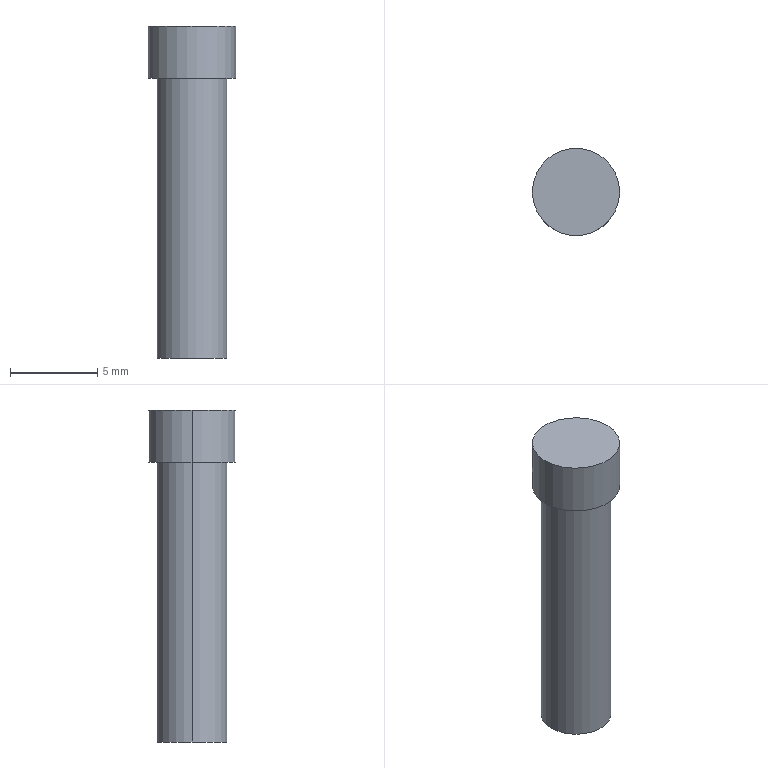Part | SolidWorks | features BaseBody 1 | 1 solid | 7 faces | box 5 x 5 x 19 mm | volume 259.967 mm3 | cylinder 4 | plane 3 | commonest cylinder face diameters 4 x2 5 x2
STEP:
#1=CARTESIAN_POINT('',(2.,0.,-5.5));
#2=VERTEX_POINT('',#1);
#3=CARTESIAN_POINT('',(-2.,0.,-5.5));
#4=VERTEX_POINT('',#3);
#5=CARTESIAN_POINT('',(0.,0.,-5.5));
#6=DIRECTION('',(0.,0.,1.));
#7=DIRECTION('',(1.,0.,0.));
#8=AXIS2_PLACEMENT_3D('',#5,#6,#7);
#9=CIRCLE('',#8,2.);
#10=EDGE_CURVE('',#2,#4,#9,.T.);
#11=ORIENTED_EDGE('',*,*,#10,.T.);
#12=CARTESIAN_POINT('',(-2.,0.,10.5));
#13=VERTEX_POINT('',#12);
#14=CARTESIAN_POINT('',(-2.,0.,-5.5));
#15=DIRECTION('',(0.,0.,1.));
#16=VECTOR('',#15,1000.);
#17=LINE('',#14,#16);
#18=EDGE_CURVE('',#4,#13,#17,.T.);
#19=ORIENTED_EDGE('',*,*,#18,.T.);
#20=CARTESIAN_POINT('',(2.,0.,10.5));
#21=VERTEX_POINT('',#20);
#22=CARTESIAN_POINT('',(0.,0.,10.5));
#23=DIRECTION('',(0.,0.,-1.));
#24=DIRECTION('',(1.,0.,0.));
#25=AXIS2_PLACEMENT_3D('',#22,#23,#24);
#26=CIRCLE('',#25,2.);
#27=EDGE_CURVE('',#13,#21,#26,.T.);
#28=ORIENTED_EDGE('',*,*,#27,.T.);
#29=CARTESIAN_POINT('',(2.,0.,-5.5));
#30=DIRECTION('',(0.,0.,1.));
#31=VECTOR('',#30,1000.);
#32=LINE('',#29,#31);
#33=EDGE_CURVE('',#2,#21,#32,.T.);
#34=ORIENTED_EDGE('',*,*,#33,.F.);
#35=EDGE_LOOP('',(#11,#19,#28,#34));
#36=FACE_OUTER_BOUND('',#35,.T.);
#37=CARTESIAN_POINT('',(0.,0.,-5.5));
#38=DIRECTION('',(0.,0.,1.));
#39=DIRECTION('',(1.,0.,0.));
#40=AXIS2_PLACEMENT_3D('',#37,#38,#39);
#41=CYLINDRICAL_SURFACE('',#40,2.);
#42=ADVANCED_FACE('',(#36),#41,.T.);
#43=CARTESIAN_POINT('',(2.5,0.,10.5));
#44=VERTEX_POINT('',#43);
#45=CARTESIAN_POINT('',(-2.5,0.,10.5));
#46=VERTEX_POINT('',#45);
#47=CARTESIAN_POINT('',(0.,0.,10.5));
#48=DIRECTION('',(0.,0.,1.));
#49=DIRECTION('',(1.,0.,0.));
#50=AXIS2_PLACEMENT_3D('',#47,#48,#49);
#51=CIRCLE('',#50,2.5);
#52=EDGE_CURVE('',#44,#46,#51,.T.);
#53=ORIENTED_EDGE('',*,*,#52,.T.);
#54=CARTESIAN_POINT('',(-2.5,0.,13.5));
#55=VERTEX_POINT('',#54);
#56=CARTESIAN_POINT('',(-2.5,0.,10.5));
#57=DIRECTION('',(0.,0.,1.));
#58=VECTOR('',#57,1000.);
#59=LINE('',#56,#58);
#60=EDGE_CURVE('',#46,#55,#59,.T.);
#61=ORIENTED_EDGE('',*,*,#60,.T.);
#62=CARTESIAN_POINT('',(2.5,0.,13.5));
#63=VERTEX_POINT('',#62);
#64=CARTESIAN_POINT('',(0.,0.,13.5));
#65=DIRECTION('',(0.,0.,-1.));
#66=DIRECTION('',(1.,0.,0.));
#67=AXIS2_PLACEMENT_3D('',#64,#65,#66);
#68=CIRCLE('',#67,2.5);
#69=EDGE_CURVE('',#55,#63,#68,.T.);
#70=ORIENTED_EDGE('',*,*,#69,.T.);
#71=CARTESIAN_POINT('',(2.5,0.,10.5));
#72=DIRECTION('',(0.,0.,1.));
#73=VECTOR('',#72,1000.);
#74=LINE('',#71,#73);
#75=EDGE_CURVE('',#44,#63,#74,.T.);
#76=ORIENTED_EDGE('',*,*,#75,.F.);
#77=EDGE_LOOP('',(#53,#61,#70,#76));
#78=FACE_OUTER_BOUND('',#77,.T.);
#79=CARTESIAN_POINT('',(0.,0.,10.5));
#80=DIRECTION('',(0.,0.,1.));
#81=DIRECTION('',(1.,0.,0.));
#82=AXIS2_PLACEMENT_3D('',#79,#80,#81);
#83=CYLINDRICAL_SURFACE('',#82,2.5);
#84=ADVANCED_FACE('',(#78),#83,.T.);
#85=ORIENTED_EDGE('',*,*,#18,.F.);
#86=CARTESIAN_POINT('',(0.,0.,-5.5));
#87=DIRECTION('',(0.,0.,1.));
#88=DIRECTION('',(1.,0.,0.));
#89=AXIS2_PLACEMENT_3D('',#86,#87,#88);
#90=CIRCLE('',#89,2.);
#91=EDGE_CURVE('',#4,#2,#90,.T.);
#92=ORIENTED_EDGE('',*,*,#91,.T.);
#93=ORIENTED_EDGE('',*,*,#33,.T.);
#94=CARTESIAN_POINT('',(0.,0.,10.5));
#95=DIRECTION('',(0.,0.,-1.));
#96=DIRECTION('',(1.,0.,0.));
#97=AXIS2_PLACEMENT_3D('',#94,#95,#96);
#98=CIRCLE('',#97,2.);
#99=EDGE_CURVE('',#21,#13,#98,.T.);
#100=ORIENTED_EDGE('',*,*,#99,.T.);
#101=EDGE_LOOP('',(#85,#92,#93,#100));
#102=FACE_OUTER_BOUND('',#101,.T.);
#103=CARTESIAN_POINT('',(0.,0.,-5.5));
#104=DIRECTION('',(0.,0.,1.));
#105=DIRECTION('',(1.,0.,0.));
#106=AXIS2_PLACEMENT_3D('',#103,#104,#105);
#107=CYLINDRICAL_SURFACE('',#106,2.);
#108=ADVANCED_FACE('',(#102),#107,.T.);
#109=ORIENTED_EDGE('',*,*,#10,.F.);
#110=ORIENTED_EDGE('',*,*,#91,.F.);
#111=EDGE_LOOP('',(#109,#110));
#112=FACE_OUTER_BOUND('',#111,.T.);
#113=CARTESIAN_POINT('',(0.,0.,-5.5));
#114=DIRECTION('',(0.,0.,1.));
#115=DIRECTION('',(1.,0.,0.));
#116=AXIS2_PLACEMENT_3D('',#113,#114,#115);
#117=PLANE('',#116);
#118=ADVANCED_FACE('',(#112),#117,.F.);
#119=ORIENTED_EDGE('',*,*,#99,.F.);
#120=ORIENTED_EDGE('',*,*,#27,.F.);
#121=EDGE_LOOP('',(#119,#120));
#122=FACE_BOUND('',#121,.T.);
#123=ORIENTED_EDGE('',*,*,#52,.F.);
#124=CARTESIAN_POINT('',(0.,0.,10.5));
#125=DIRECTION('',(0.,0.,1.));
#126=DIRECTION('',(1.,0.,0.));
#127=AXIS2_PLACEMENT_3D('',#124,#125,#126);
#128=CIRCLE('',#127,2.5);
#129=EDGE_CURVE('',#46,#44,#128,.T.);
#130=ORIENTED_EDGE('',*,*,#129,.F.);
#131=EDGE_LOOP('',(#123,#130));
#132=FACE_OUTER_BOUND('',#131,.T.);
#133=CARTESIAN_POINT('',(0.,0.,10.5));
#134=DIRECTION('',(0.,0.,1.));
#135=DIRECTION('',(1.,0.,0.));
#136=AXIS2_PLACEMENT_3D('',#133,#134,#135);
#137=PLANE('',#136);
#138=ADVANCED_FACE('',(#122,#132),#137,.F.);
#139=ORIENTED_EDGE('',*,*,#60,.F.);
#140=ORIENTED_EDGE('',*,*,#129,.T.);
#141=ORIENTED_EDGE('',*,*,#75,.T.);
#142=CARTESIAN_POINT('',(0.,0.,13.5));
#143=DIRECTION('',(0.,0.,-1.));
#144=DIRECTION('',(1.,0.,0.));
#145=AXIS2_PLACEMENT_3D('',#142,#143,#144);
#146=CIRCLE('',#145,2.5);
#147=EDGE_CURVE('',#63,#55,#146,.T.);
#148=ORIENTED_EDGE('',*,*,#147,.T.);
#149=EDGE_LOOP('',(#139,#140,#141,#148));
#150=FACE_OUTER_BOUND('',#149,.T.);
#151=CARTESIAN_POINT('',(0.,0.,10.5));
#152=DIRECTION('',(0.,0.,1.));
#153=DIRECTION('',(1.,0.,0.));
#154=AXIS2_PLACEMENT_3D('',#151,#152,#153);
#155=CYLINDRICAL_SURFACE('',#154,2.5);
#156=ADVANCED_FACE('',(#150),#155,.T.);
#157=ORIENTED_EDGE('',*,*,#147,.F.);
#158=ORIENTED_EDGE('',*,*,#69,.F.);
#159=EDGE_LOOP('',(#157,#158));
#160=FACE_OUTER_BOUND('',#159,.T.);
#161=CARTESIAN_POINT('',(0.,0.,13.5));
#162=DIRECTION('',(0.,0.,1.));
#163=DIRECTION('',(1.,0.,0.));
#164=AXIS2_PLACEMENT_3D('',#161,#162,#163);
#165=PLANE('',#164);
#166=ADVANCED_FACE('',(#160),#165,.T.);
#167=CLOSED_SHELL('',(#42,#84,#108,#118,#138,#156,#166));
#168=MANIFOLD_SOLID_BREP('',#167);
#169=CARTESIAN_POINT('',(0.,0.,0.));
#170=DIRECTION('',(0.,0.,1.));
#171=DIRECTION('',(1.,0.,0.));
#172=AXIS2_PLACEMENT_3D('',#169,#170,#171);
#173=(LENGTH_UNIT()NAMED_UNIT(*)SI_UNIT(.MILLI.,.METRE.));
#174=UNCERTAINTY_MEASURE_WITH_UNIT(LENGTH_MEASURE(0.00001),#173,'','');
#175=(NAMED_UNIT(*)PLANE_ANGLE_UNIT()SI_UNIT($,.RADIAN.));
#176=(NAMED_UNIT(*)SI_UNIT($,.STERADIAN.)SOLID_ANGLE_UNIT());
#177=(GEOMETRIC_REPRESENTATION_CONTEXT(3)GLOBAL_UNCERTAINTY_ASSIGNED_CONTEXT((#174))GLOBAL_UNIT_ASSIGNED_CONTEXT((#173,#175,#176))REPRESENTATION_CONTEXT('',''));
#178=ADVANCED_BREP_SHAPE_REPRESENTATION('',(#168,#172),#177);